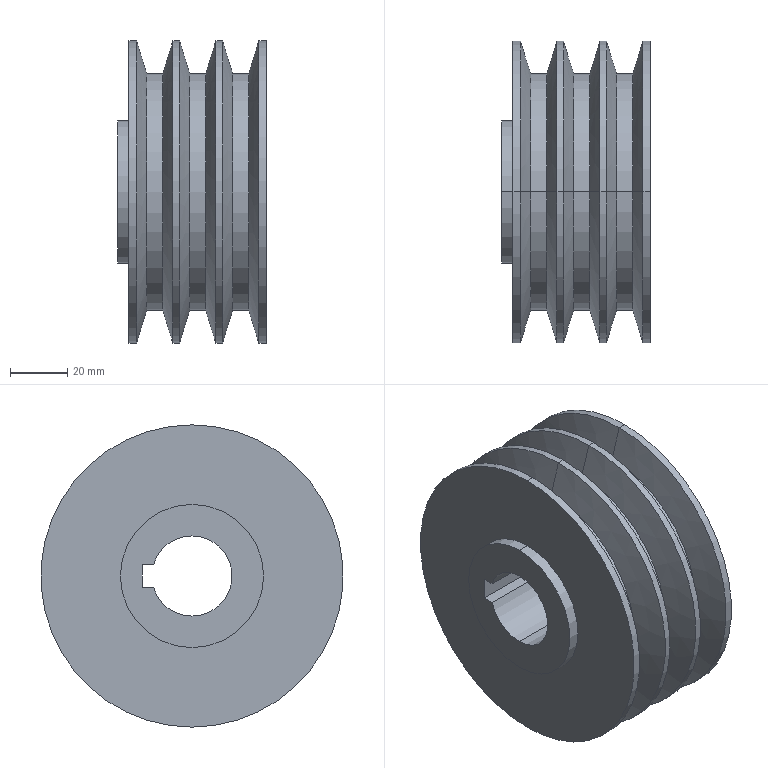Part | SolidWorks | features ICE 2, Revolution 1 | 1 solid | 37 faces | box 52 x 105.5 x 105.5 mm | volume 299364 mm3 | cylinder 19 | cone 12 | plane 6 | commonest cylinder face diameters 105.5 x8 82.6 x6 28 x3 50 x2
STEP:
#1=CARTESIAN_POINT('',(-4.,0.,25.));
#2=VERTEX_POINT('',#1);
#3=CARTESIAN_POINT('',(-4.,0.,-25.));
#4=VERTEX_POINT('',#3);
#5=CARTESIAN_POINT('',(-4.,0.,0.));
#6=DIRECTION('',(-1.,0.,0.));
#7=DIRECTION('',(0.,0.,1.));
#8=AXIS2_PLACEMENT_3D('',#5,#6,#7);
#9=CIRCLE('',#8,25.);
#10=EDGE_CURVE('',#2,#4,#9,.T.);
#11=ORIENTED_EDGE('',*,*,#10,.F.);
#12=CARTESIAN_POINT('',(0.,0.,25.));
#13=VERTEX_POINT('',#12);
#14=CARTESIAN_POINT('',(-4.,0.,25.));
#15=DIRECTION('',(1.,0.,0.));
#16=VECTOR('',#15,1000.);
#17=LINE('',#14,#16);
#18=EDGE_CURVE('',#2,#13,#17,.T.);
#19=ORIENTED_EDGE('',*,*,#18,.T.);
#20=CARTESIAN_POINT('',(0.,0.,-25.));
#21=VERTEX_POINT('',#20);
#22=CARTESIAN_POINT('',(0.,0.,0.));
#23=DIRECTION('',(-1.,0.,0.));
#24=DIRECTION('',(0.,0.,1.));
#25=AXIS2_PLACEMENT_3D('',#22,#23,#24);
#26=CIRCLE('',#25,25.);
#27=EDGE_CURVE('',#13,#21,#26,.T.);
#28=ORIENTED_EDGE('',*,*,#27,.T.);
#29=CARTESIAN_POINT('',(-4.,0.,-25.));
#30=DIRECTION('',(1.,0.,0.));
#31=VECTOR('',#30,1000.);
#32=LINE('',#29,#31);
#33=EDGE_CURVE('',#4,#21,#32,.T.);
#34=ORIENTED_EDGE('',*,*,#33,.F.);
#35=EDGE_LOOP('',(#11,#19,#28,#34));
#36=FACE_OUTER_BOUND('',#35,.T.);
#37=CARTESIAN_POINT('',(-4.,0.,0.));
#38=DIRECTION('',(1.,0.,0.));
#39=DIRECTION('',(0.,0.,-1.));
#40=AXIS2_PLACEMENT_3D('',#37,#38,#39);
#41=CYLINDRICAL_SURFACE('',#40,25.);
#42=ADVANCED_FACE('',(#36),#41,.T.);
#43=CARTESIAN_POINT('',(11.839,0.,-41.3));
#44=VERTEX_POINT('',#43);
#45=CARTESIAN_POINT('',(11.839,0.,41.3));
#46=VERTEX_POINT('',#45);
#47=CARTESIAN_POINT('',(11.839,0.,0.));
#48=DIRECTION('',(1.,0.,0.));
#49=DIRECTION('',(0.,0.,-1.));
#50=AXIS2_PLACEMENT_3D('',#47,#48,#49);
#51=CIRCLE('',#50,41.3);
#52=EDGE_CURVE('',#44,#46,#51,.T.);
#53=ORIENTED_EDGE('',*,*,#52,.T.);
#54=CARTESIAN_POINT('',(15.339,0.,52.75));
#55=VERTEX_POINT('',#54);
#56=CARTESIAN_POINT('',(15.339,0.,52.75));
#57=DIRECTION('',(0.2924,0.,0.9563));
#58=VECTOR('',#57,1000.);
#59=LINE('',#56,#58);
#60=EDGE_CURVE('',#46,#55,#59,.T.);
#61=ORIENTED_EDGE('',*,*,#60,.T.);
#62=CARTESIAN_POINT('',(15.339,0.,-52.75));
#63=VERTEX_POINT('',#62);
#64=CARTESIAN_POINT('',(15.339,0.,0.));
#65=DIRECTION('',(1.,0.,0.));
#66=DIRECTION('',(0.,0.,-1.));
#67=AXIS2_PLACEMENT_3D('',#64,#65,#66);
#68=CIRCLE('',#67,52.75);
#69=EDGE_CURVE('',#63,#55,#68,.T.);
#70=ORIENTED_EDGE('',*,*,#69,.F.);
#71=CARTESIAN_POINT('',(15.339,0.,-52.75));
#72=DIRECTION('',(0.2924,0.,-0.9563));
#73=VECTOR('',#72,1000.);
#74=LINE('',#71,#73);
#75=EDGE_CURVE('',#44,#63,#74,.T.);
#76=ORIENTED_EDGE('',*,*,#75,.F.);
#77=EDGE_LOOP('',(#53,#61,#70,#76));
#78=FACE_OUTER_BOUND('',#77,.T.);
#79=CARTESIAN_POINT('',(15.339,0.,0.));
#80=DIRECTION('',(1.,0.,0.));
#81=DIRECTION('',(0.,0.,-1.));
#82=AXIS2_PLACEMENT_3D('',#79,#80,#81);
#83=CONICAL_SURFACE('',#82,52.75,1.274);
#84=ADVANCED_FACE('',(#78),#83,.T.);
#85=ORIENTED_EDGE('',*,*,#69,.T.);
#86=CARTESIAN_POINT('',(17.659,0.,52.75));
#87=VERTEX_POINT('',#86);
#88=CARTESIAN_POINT('',(0.,0.,52.75));
#89=DIRECTION('',(1.,0.,0.));
#90=VECTOR('',#89,1000.);
#91=LINE('',#88,#90);
#92=EDGE_CURVE('',#55,#87,#91,.T.);
#93=ORIENTED_EDGE('',*,*,#92,.T.);
#94=CARTESIAN_POINT('',(17.659,0.,-52.75));
#95=VERTEX_POINT('',#94);
#96=CARTESIAN_POINT('',(17.659,0.,0.));
#97=DIRECTION('',(1.,0.,0.));
#98=DIRECTION('',(0.,0.,-1.));
#99=AXIS2_PLACEMENT_3D('',#96,#97,#98);
#100=CIRCLE('',#99,52.75);
#101=EDGE_CURVE('',#95,#87,#100,.T.);
#102=ORIENTED_EDGE('',*,*,#101,.F.);
#103=CARTESIAN_POINT('',(0.,0.,-52.75));
#104=DIRECTION('',(1.,0.,0.));
#105=VECTOR('',#104,1000.);
#106=LINE('',#103,#105);
#107=EDGE_CURVE('',#63,#95,#106,.T.);
#108=ORIENTED_EDGE('',*,*,#107,.F.);
#109=EDGE_LOOP('',(#85,#93,#102,#108));
#110=FACE_OUTER_BOUND('',#109,.T.);
#111=CARTESIAN_POINT('',(0.,0.,0.));
#112=DIRECTION('',(1.,0.,0.));
#113=DIRECTION('',(0.,0.,-1.));
#114=AXIS2_PLACEMENT_3D('',#111,#112,#113);
#115=CYLINDRICAL_SURFACE('',#114,52.75);
#116=ADVANCED_FACE('',(#110),#115,.T.);
#117=CARTESIAN_POINT('',(21.16,0.,-41.3));
#118=VERTEX_POINT('',#117);
#119=CARTESIAN_POINT('',(21.16,0.,41.3));
#120=VERTEX_POINT('',#119);
#121=CARTESIAN_POINT('',(21.16,0.,0.));
#122=DIRECTION('',(1.,0.,0.));
#123=DIRECTION('',(0.,0.,-1.));
#124=AXIS2_PLACEMENT_3D('',#121,#122,#123);
#125=CIRCLE('',#124,41.3);
#126=EDGE_CURVE('',#118,#120,#125,.T.);
#127=ORIENTED_EDGE('',*,*,#126,.F.);
#128=CARTESIAN_POINT('',(21.16,0.,-41.3));
#129=DIRECTION('',(-0.2924,0.,-0.9563));
#130=VECTOR('',#129,1000.);
#131=LINE('',#128,#130);
#132=EDGE_CURVE('',#118,#95,#131,.T.);
#133=ORIENTED_EDGE('',*,*,#132,.T.);
#134=ORIENTED_EDGE('',*,*,#101,.T.);
#135=CARTESIAN_POINT('',(21.16,0.,41.3));
#136=DIRECTION('',(-0.2924,0.,0.9563));
#137=VECTOR('',#136,1000.);
#138=LINE('',#135,#137);
#139=EDGE_CURVE('',#120,#87,#138,.T.);
#140=ORIENTED_EDGE('',*,*,#139,.F.);
#141=EDGE_LOOP('',(#127,#133,#134,#140));
#142=FACE_OUTER_BOUND('',#141,.T.);
#143=CARTESIAN_POINT('',(21.16,0.,0.));
#144=DIRECTION('',(-1.,0.,0.));
#145=DIRECTION('',(0.,0.,1.));
#146=AXIS2_PLACEMENT_3D('',#143,#144,#145);
#147=CONICAL_SURFACE('',#146,41.3,1.274);
#148=ADVANCED_FACE('',(#142),#147,.T.);
#149=ORIENTED_EDGE('',*,*,#126,.T.);
#150=CARTESIAN_POINT('',(26.84,0.,41.3));
#151=VERTEX_POINT('',#150);
#152=CARTESIAN_POINT('',(0.,0.,41.3));
#153=DIRECTION('',(1.,0.,0.));
#154=VECTOR('',#153,1000.);
#155=LINE('',#152,#154);
#156=EDGE_CURVE('',#120,#151,#155,.T.);
#157=ORIENTED_EDGE('',*,*,#156,.T.);
#158=CARTESIAN_POINT('',(26.84,0.,-41.3));
#159=VERTEX_POINT('',#158);
#160=CARTESIAN_POINT('',(26.84,0.,0.));
#161=DIRECTION('',(1.,0.,0.));
#162=DIRECTION('',(0.,0.,-1.));
#163=AXIS2_PLACEMENT_3D('',#160,#161,#162);
#164=CIRCLE('',#163,41.3);
#165=EDGE_CURVE('',#159,#151,#164,.T.);
#166=ORIENTED_EDGE('',*,*,#165,.F.);
#167=CARTESIAN_POINT('',(0.,0.,-41.3));
#168=DIRECTION('',(1.,0.,0.));
#169=VECTOR('',#168,1000.);
#170=LINE('',#167,#169);
#171=EDGE_CURVE('',#118,#159,#170,.T.);
#172=ORIENTED_EDGE('',*,*,#171,.F.);
#173=EDGE_LOOP('',(#149,#157,#166,#172));
#174=FACE_OUTER_BOUND('',#173,.T.);
#175=CARTESIAN_POINT('',(0.,0.,0.));
#176=DIRECTION('',(1.,0.,0.));
#177=DIRECTION('',(0.,0.,-1.));
#178=AXIS2_PLACEMENT_3D('',#175,#176,#177);
#179=CYLINDRICAL_SURFACE('',#178,41.3);
#180=ADVANCED_FACE('',(#174),#179,.T.);
#181=ORIENTED_EDGE('',*,*,#165,.T.);
#182=CARTESIAN_POINT('',(30.341,0.,52.75));
#183=VERTEX_POINT('',#182);
#184=CARTESIAN_POINT('',(30.341,0.,52.75));
#185=DIRECTION('',(0.2924,0.,0.9563));
#186=VECTOR('',#185,1000.);
#187=LINE('',#184,#186);
#188=EDGE_CURVE('',#151,#183,#187,.T.);
#189=ORIENTED_EDGE('',*,*,#188,.T.);
#190=CARTESIAN_POINT('',(30.341,0.,-52.75));
#191=VERTEX_POINT('',#190);
#192=CARTESIAN_POINT('',(30.341,0.,0.));
#193=DIRECTION('',(1.,0.,0.));
#194=DIRECTION('',(0.,0.,-1.));
#195=AXIS2_PLACEMENT_3D('',#192,#193,#194);
#196=CIRCLE('',#195,52.75);
#197=EDGE_CURVE('',#191,#183,#196,.T.);
#198=ORIENTED_EDGE('',*,*,#197,.F.);
#199=CARTESIAN_POINT('',(30.341,0.,-52.75));
#200=DIRECTION('',(0.2924,0.,-0.9563));
#201=VECTOR('',#200,1000.);
#202=LINE('',#199,#201);
#203=EDGE_CURVE('',#159,#191,#202,.T.);
#204=ORIENTED_EDGE('',*,*,#203,.F.);
#205=EDGE_LOOP('',(#181,#189,#198,#204));
#206=FACE_OUTER_BOUND('',#205,.T.);
#207=CARTESIAN_POINT('',(30.341,0.,0.));
#208=DIRECTION('',(1.,0.,0.));
#209=DIRECTION('',(0.,0.,-1.));
#210=AXIS2_PLACEMENT_3D('',#207,#208,#209);
#211=CONICAL_SURFACE('',#210,52.75,1.274);
#212=ADVANCED_FACE('',(#206),#211,.T.);
#213=ORIENTED_EDGE('',*,*,#197,.T.);
#214=CARTESIAN_POINT('',(32.661,0.,52.75));
#215=VERTEX_POINT('',#214);
#216=CARTESIAN_POINT('',(0.,0.,52.75));
#217=DIRECTION('',(1.,0.,0.));
#218=VECTOR('',#217,1000.);
#219=LINE('',#216,#218);
#220=EDGE_CURVE('',#183,#215,#219,.T.);
#221=ORIENTED_EDGE('',*,*,#220,.T.);
#222=CARTESIAN_POINT('',(32.661,0.,-52.75));
#223=VERTEX_POINT('',#222);
#224=CARTESIAN_POINT('',(32.661,0.,0.));
#225=DIRECTION('',(1.,0.,0.));
#226=DIRECTION('',(0.,0.,-1.));
#227=AXIS2_PLACEMENT_3D('',#224,#225,#226);
#228=CIRCLE('',#227,52.75);
#229=EDGE_CURVE('',#223,#215,#228,.T.);
#230=ORIENTED_EDGE('',*,*,#229,.F.);
#231=CARTESIAN_POINT('',(0.,0.,-52.75));
#232=DIRECTION('',(1.,0.,0.));
#233=VECTOR('',#232,1000.);
#234=LINE('',#231,#233);
#235=EDGE_CURVE('',#191,#223,#234,.T.);
#236=ORIENTED_EDGE('',*,*,#235,.F.);
#237=EDGE_LOOP('',(#213,#221,#230,#236));
#238=FACE_OUTER_BOUND('',#237,.T.);
#239=CARTESIAN_POINT('',(0.,0.,0.));
#240=DIRECTION('',(1.,0.,0.));
#241=DIRECTION('',(0.,0.,-1.));
#242=AXIS2_PLACEMENT_3D('',#239,#240,#241);
#243=CYLINDRICAL_SURFACE('',#242,52.75);
#244=ADVANCED_FACE('',(#238),#243,.T.);
#245=CARTESIAN_POINT('',(36.161,0.,-41.3));
#246=VERTEX_POINT('',#245);
#247=CARTESIAN_POINT('',(36.161,0.,41.3));
#248=VERTEX_POINT('',#247);
#249=CARTESIAN_POINT('',(36.161,0.,0.));
#250=DIRECTION('',(1.,0.,0.));
#251=DIRECTION('',(0.,0.,-1.));
#252=AXIS2_PLACEMENT_3D('',#249,#250,#251);
#253=CIRCLE('',#252,41.3);
#254=EDGE_CURVE('',#246,#248,#253,.T.);
#255=ORIENTED_EDGE('',*,*,#254,.F.);
#256=CARTESIAN_POINT('',(36.161,0.,-41.3));
#257=DIRECTION('',(-0.2924,0.,-0.9563));
#258=VECTOR('',#257,1000.);
#259=LINE('',#256,#258);
#260=EDGE_CURVE('',#246,#223,#259,.T.);
#261=ORIENTED_EDGE('',*,*,#260,.T.);
#262=ORIENTED_EDGE('',*,*,#229,.T.);
#263=CARTESIAN_POINT('',(36.161,0.,41.3));
#264=DIRECTION('',(-0.2924,0.,0.9563));
#265=VECTOR('',#264,1000.);
#266=LINE('',#263,#265);
#267=EDGE_CURVE('',#248,#215,#266,.T.);
#268=ORIENTED_EDGE('',*,*,#267,.F.);
#269=EDGE_LOOP('',(#255,#261,#262,#268));
#270=FACE_OUTER_BOUND('',#269,.T.);
#271=CARTESIAN_POINT('',(36.161,0.,0.));
#272=DIRECTION('',(-1.,0.,0.));
#273=DIRECTION('',(0.,0.,1.));
#274=AXIS2_PLACEMENT_3D('',#271,#272,#273);
#275=CONICAL_SURFACE('',#274,41.3,1.274);
#276=ADVANCED_FACE('',(#270),#275,.T.);
#277=ORIENTED_EDGE('',*,*,#254,.T.);
#278=CARTESIAN_POINT('',(41.841,0.,41.3));
#279=VERTEX_POINT('',#278);
#280=CARTESIAN_POINT('',(0.,0.,41.3));
#281=DIRECTION('',(1.,0.,0.));
#282=VECTOR('',#281,1000.);
#283=LINE('',#280,#282);
#284=EDGE_CURVE('',#248,#279,#283,.T.);
#285=ORIENTED_EDGE('',*,*,#284,.T.);
#286=CARTESIAN_POINT('',(41.841,0.,-41.3));
#287=VERTEX_POINT('',#286);
#288=CARTESIAN_POINT('',(41.841,0.,0.));
#289=DIRECTION('',(1.,0.,0.));
#290=DIRECTION('',(0.,0.,-1.));
#291=AXIS2_PLACEMENT_3D('',#288,#289,#290);
#292=CIRCLE('',#291,41.3);
#293=EDGE_CURVE('',#287,#279,#292,.T.);
#294=ORIENTED_EDGE('',*,*,#293,.F.);
#295=CARTESIAN_POINT('',(0.,0.,-41.3));
#296=DIRECTION('',(1.,0.,0.));
#297=VECTOR('',#296,1000.);
#298=LINE('',#295,#297);
#299=EDGE_CURVE('',#246,#287,#298,.T.);
#300=ORIENTED_EDGE('',*,*,#299,.F.);
#301=EDGE_LOOP('',(#277,#285,#294,#300));
#302=FACE_OUTER_BOUND('',#301,.T.);
#303=CARTESIAN_POINT('',(0.,0.,0.));
#304=DIRECTION('',(1.,0.,0.));
#305=DIRECTION('',(0.,0.,-1.));
#306=AXIS2_PLACEMENT_3D('',#303,#304,#305);
#307=CYLINDRICAL_SURFACE('',#306,41.3);
#308=ADVANCED_FACE('',(#302),#307,.T.);
#309=ORIENTED_EDGE('',*,*,#293,.T.);
#310=CARTESIAN_POINT('',(45.342,0.,52.75));
#311=VERTEX_POINT('',#310);
#312=CARTESIAN_POINT('',(45.342,0.,52.75));
#313=DIRECTION('',(0.2924,0.,0.9563));
#314=VECTOR('',#313,1000.);
#315=LINE('',#312,#314);
#316=EDGE_CURVE('',#279,#311,#315,.T.);
#317=ORIENTED_EDGE('',*,*,#316,.T.);
#318=CARTESIAN_POINT('',(45.342,0.,-52.75));
#319=VERTEX_POINT('',#318);
#320=CARTESIAN_POINT('',(45.342,0.,0.));
#321=DIRECTION('',(1.,0.,0.));
#322=DIRECTION('',(0.,0.,-1.));
#323=AXIS2_PLACEMENT_3D('',#320,#321,#322);
#324=CIRCLE('',#323,52.75);
#325=EDGE_CURVE('',#319,#311,#324,.T.);
#326=ORIENTED_EDGE('',*,*,#325,.F.);
#327=CARTESIAN_POINT('',(45.342,0.,-52.75));
#328=DIRECTION('',(0.2924,0.,-0.9563));
#329=VECTOR('',#328,1000.);
#330=LINE('',#327,#329);
#331=EDGE_CURVE('',#287,#319,#330,.T.);
#332=ORIENTED_EDGE('',*,*,#331,.F.);
#333=EDGE_LOOP('',(#309,#317,#326,#332));
#334=FACE_OUTER_BOUND('',#333,.T.);
#335=CARTESIAN_POINT('',(45.342,0.,0.));
#336=DIRECTION('',(1.,0.,0.));
#337=DIRECTION('',(0.,0.,-1.));
#338=AXIS2_PLACEMENT_3D('',#335,#336,#337);
#339=CONICAL_SURFACE('',#338,52.75,1.274);
#340=ADVANCED_FACE('',(#334),#339,.T.);
#341=ORIENTED_EDGE('',*,*,#325,.T.);
#342=CARTESIAN_POINT('',(48.,0.,52.75));
#343=VERTEX_POINT('',#342);
#344=CARTESIAN_POINT('',(0.,0.,52.75));
#345=DIRECTION('',(1.,0.,0.));
#346=VECTOR('',#345,1000.);
#347=LINE('',#344,#346);
#348=EDGE_CURVE('',#311,#343,#347,.T.);
#349=ORIENTED_EDGE('',*,*,#348,.T.);
#350=CARTESIAN_POINT('',(48.,0.,-52.75));
#351=VERTEX_POINT('',#350);
#352=CARTESIAN_POINT('',(48.,0.,0.));
#353=DIRECTION('',(1.,0.,0.));
#354=DIRECTION('',(0.,0.,-1.));
#355=AXIS2_PLACEMENT_3D('',#352,#353,#354);
#356=CIRCLE('',#355,52.75);
#357=EDGE_CURVE('',#351,#343,#356,.T.);
#358=ORIENTED_EDGE('',*,*,#357,.F.);
#359=CARTESIAN_POINT('',(0.,0.,-52.75));
#360=DIRECTION('',(1.,0.,0.));
#361=VECTOR('',#360,1000.);
#362=LINE('',#359,#361);
#363=EDGE_CURVE('',#319,#351,#362,.T.);
#364=ORIENTED_EDGE('',*,*,#363,.F.);
#365=EDGE_LOOP('',(#341,#349,#358,#364));
#366=FACE_OUTER_BOUND('',#365,.T.);
#367=CARTESIAN_POINT('',(0.,0.,0.));
#368=DIRECTION('',(1.,0.,0.));
#369=DIRECTION('',(0.,0.,-1.));
#370=AXIS2_PLACEMENT_3D('',#367,#368,#369);
#371=CYLINDRICAL_SURFACE('',#370,52.75);
#372=ADVANCED_FACE('',(#366),#371,.T.);
#373=CARTESIAN_POINT('',(-4.,0.,-14.));
#374=VERTEX_POINT('',#373);
#375=CARTESIAN_POINT('',(-4.,0.,14.));
#376=VERTEX_POINT('',#375);
#377=CARTESIAN_POINT('',(-4.,0.,0.));
#378=DIRECTION('',(-1.,0.,0.));
#379=DIRECTION('',(0.,0.,1.));
#380=AXIS2_PLACEMENT_3D('',#377,#378,#379);
#381=CIRCLE('',#380,14.);
#382=EDGE_CURVE('',#374,#376,#381,.T.);
#383=ORIENTED_EDGE('',*,*,#382,.T.);
#384=CARTESIAN_POINT('',(48.,0.,14.));
#385=VERTEX_POINT('',#384);
#386=CARTESIAN_POINT('',(0.,0.,14.));
#387=DIRECTION('',(1.,0.,0.));
#388=VECTOR('',#387,1000.);
#389=LINE('',#386,#388);
#390=EDGE_CURVE('',#376,#385,#389,.T.);
#391=ORIENTED_EDGE('',*,*,#390,.T.);
#392=CARTESIAN_POINT('',(48.,0.,-14.));
#393=VERTEX_POINT('',#392);
#394=CARTESIAN_POINT('',(48.,0.,0.));
#395=DIRECTION('',(1.,0.,0.));
#396=DIRECTION('',(0.,0.,-1.));
#397=AXIS2_PLACEMENT_3D('',#394,#395,#396);
#398=CIRCLE('',#397,14.);
#399=EDGE_CURVE('',#385,#393,#398,.T.);
#400=ORIENTED_EDGE('',*,*,#399,.T.);
#401=CARTESIAN_POINT('',(0.,0.,-14.));
#402=DIRECTION('',(1.,0.,0.));
#403=VECTOR('',#402,1000.);
#404=LINE('',#401,#403);
#405=EDGE_CURVE('',#374,#393,#404,.T.);
#406=ORIENTED_EDGE('',*,*,#405,.F.);
#407=EDGE_LOOP('',(#383,#391,#400,#406));
#408=FACE_OUTER_BOUND('',#407,.T.);
#409=CARTESIAN_POINT('',(0.,0.,0.));
#410=DIRECTION('',(1.,0.,0.));
#411=DIRECTION('',(0.,0.,-1.));
#412=AXIS2_PLACEMENT_3D('',#409,#410,#411);
#413=CYLINDRICAL_SURFACE('',#412,14.);
#414=ADVANCED_FACE('',(#408),#413,.F.);
#415=CARTESIAN_POINT('',(-4.,13.416,-4.));
#416=VERTEX_POINT('',#415);
#417=CARTESIAN_POINT('',(-4.,0.,0.));
#418=DIRECTION('',(-1.,0.,0.));
#419=DIRECTION('',(0.,0.,1.));
#420=AXIS2_PLACEMENT_3D('',#417,#418,#419);
#421=CIRCLE('',#420,14.);
#422=EDGE_CURVE('',#416,#374,#421,.T.);
#423=ORIENTED_EDGE('',*,*,#422,.T.);
#424=ORIENTED_EDGE('',*,*,#405,.T.);
#425=CARTESIAN_POINT('',(48.,13.416,-4.));
#426=VERTEX_POINT('',#425);
#427=CARTESIAN_POINT('',(48.,0.,0.));
#428=DIRECTION('',(1.,0.,0.));
#429=DIRECTION('',(0.,0.,-1.));
#430=AXIS2_PLACEMENT_3D('',#427,#428,#429);
#431=CIRCLE('',#430,14.);
#432=EDGE_CURVE('',#393,#426,#431,.T.);
#433=ORIENTED_EDGE('',*,*,#432,.T.);
#434=CARTESIAN_POINT('',(0.,13.416,-4.));
#435=DIRECTION('',(-1.,0.,0.));
#436=VECTOR('',#435,1000.);
#437=LINE('',#434,#436);
#438=EDGE_CURVE('',#426,#416,#437,.T.);
#439=ORIENTED_EDGE('',*,*,#438,.T.);
#440=EDGE_LOOP('',(#423,#424,#433,#439));
#441=FACE_OUTER_BOUND('',#440,.T.);
#442=CARTESIAN_POINT('',(0.,0.,0.));
#443=DIRECTION('',(1.,0.,0.));
#444=DIRECTION('',(0.,0.,-1.));
#445=AXIS2_PLACEMENT_3D('',#442,#443,#444);
#446=CYLINDRICAL_SURFACE('',#445,14.);
#447=ADVANCED_FACE('',(#441),#446,.F.);
#448=CARTESIAN_POINT('',(0.,0.,-52.75));
#449=VERTEX_POINT('',#448);
#450=CARTESIAN_POINT('',(0.,0.,52.75));
#451=VERTEX_POINT('',#450);
#452=CARTESIAN_POINT('',(0.,0.,0.));
#453=DIRECTION('',(1.,0.,0.));
#454=DIRECTION('',(0.,0.,-1.));
#455=AXIS2_PLACEMENT_3D('',#452,#453,#454);
#456=CIRCLE('',#455,52.75);
#457=EDGE_CURVE('',#449,#451,#456,.T.);
#458=ORIENTED_EDGE('',*,*,#457,.T.);
#459=CARTESIAN_POINT('',(2.658,0.,52.75));
#460=VERTEX_POINT('',#459);
#461=CARTESIAN_POINT('',(0.,0.,52.75));
#462=DIRECTION('',(1.,0.,0.));
#463=VECTOR('',#462,1000.);
#464=LINE('',#461,#463);
#465=EDGE_CURVE('',#451,#460,#464,.T.);
#466=ORIENTED_EDGE('',*,*,#465,.T.);
#467=CARTESIAN_POINT('',(2.658,0.,-52.75));
#468=VERTEX_POINT('',#467);
#469=CARTESIAN_POINT('',(2.658,0.,0.));
#470=DIRECTION('',(1.,0.,0.));
#471=DIRECTION('',(0.,0.,-1.));
#472=AXIS2_PLACEMENT_3D('',#469,#470,#471);
#473=CIRCLE('',#472,52.75);
#474=EDGE_CURVE('',#468,#460,#473,.T.);
#475=ORIENTED_EDGE('',*,*,#474,.F.);
#476=CARTESIAN_POINT('',(0.,0.,-52.75));
#477=DIRECTION('',(1.,0.,0.));
#478=VECTOR('',#477,1000.);
#479=LINE('',#476,#478);
#480=EDGE_CURVE('',#449,#468,#479,.T.);
#481=ORIENTED_EDGE('',*,*,#480,.F.);
#482=EDGE_LOOP('',(#458,#466,#475,#481));
#483=FACE_OUTER_BOUND('',#482,.T.);
#484=CARTESIAN_POINT('',(0.,0.,0.));
#485=DIRECTION('',(1.,0.,0.));
#486=DIRECTION('',(0.,0.,-1.));
#487=AXIS2_PLACEMENT_3D('',#484,#485,#486);
#488=CYLINDRICAL_SURFACE('',#487,52.75);
#489=ADVANCED_FACE('',(#483),#488,.T.);
#490=CARTESIAN_POINT('',(6.159,0.,-41.3));
#491=VERTEX_POINT('',#490);
#492=CARTESIAN_POINT('',(6.159,0.,41.3));
#493=VERTEX_POINT('',#492);
#494=CARTESIAN_POINT('',(6.159,0.,0.));
#495=DIRECTION('',(1.,0.,0.));
#496=DIRECTION('',(0.,0.,-1.));
#497=AXIS2_PLACEMENT_3D('',#494,#495,#496);
#498=CIRCLE('',#497,41.3);
#499=EDGE_CURVE('',#491,#493,#498,.T.);
#500=ORIENTED_EDGE('',*,*,#499,.F.);
#501=CARTESIAN_POINT('',(6.159,0.,-41.3));
#502=DIRECTION('',(-0.2924,0.,-0.9563));
#503=VECTOR('',#502,1000.);
#504=LINE('',#501,#503);
#505=EDGE_CURVE('',#491,#468,#504,.T.);
#506=ORIENTED_EDGE('',*,*,#505,.T.);
#507=ORIENTED_EDGE('',*,*,#474,.T.);
#508=CARTESIAN_POINT('',(6.159,0.,41.3));
#509=DIRECTION('',(-0.2924,0.,0.9563));
#510=VECTOR('',#509,1000.);
#511=LINE('',#508,#510);
#512=EDGE_CURVE('',#493,#460,#511,.T.);
#513=ORIENTED_EDGE('',*,*,#512,.F.);
#514=EDGE_LOOP('',(#500,#506,#507,#513));
#515=FACE_OUTER_BOUND('',#514,.T.);
#516=CARTESIAN_POINT('',(6.159,0.,0.));
#517=DIRECTION('',(-1.,0.,0.));
#518=DIRECTION('',(0.,0.,1.));
#519=AXIS2_PLACEMENT_3D('',#516,#517,#518);
#520=CONICAL_SURFACE('',#519,41.3,1.274);
#521=ADVANCED_FACE('',(#515),#520,.T.);
#522=ORIENTED_EDGE('',*,*,#499,.T.);
#523=CARTESIAN_POINT('',(0.,0.,41.3));
#524=DIRECTION('',(1.,0.,0.));
#525=VECTOR('',#524,1000.);
#526=LINE('',#523,#525);
#527=EDGE_CURVE('',#493,#46,#526,.T.);
#528=ORIENTED_EDGE('',*,*,#527,.T.);
#529=ORIENTED_EDGE('',*,*,#52,.F.);
#530=CARTESIAN_POINT('',(0.,0.,-41.3));
#531=DIRECTION('',(1.,0.,0.));
#532=VECTOR('',#531,1000.);
#533=LINE('',#530,#532);
#534=EDGE_CURVE('',#491,#44,#533,.T.);
#535=ORIENTED_EDGE('',*,*,#534,.F.);
#536=EDGE_LOOP('',(#522,#528,#529,#535));
#537=FACE_OUTER_BOUND('',#536,.T.);
#538=CARTESIAN_POINT('',(0.,0.,0.));
#539=DIRECTION('',(1.,0.,0.));
#540=DIRECTION('',(0.,0.,-1.));
#541=AXIS2_PLACEMENT_3D('',#538,#539,#540);
#542=CYLINDRICAL_SURFACE('',#541,41.3);
#543=ADVANCED_FACE('',(#537),#542,.T.);
#544=ORIENTED_EDGE('',*,*,#457,.F.);
#545=CARTESIAN_POINT('',(0.,0.,0.));
#546=DIRECTION('',(1.,0.,0.));
#547=DIRECTION('',(0.,0.,-1.));
#548=AXIS2_PLACEMENT_3D('',#545,#546,#547);
#549=CIRCLE('',#548,52.75);
#550=EDGE_CURVE('',#451,#449,#549,.T.);
#551=ORIENTED_EDGE('',*,*,#550,.F.);
#552=EDGE_LOOP('',(#544,#551));
#553=FACE_OUTER_BOUND('',#552,.T.);
#554=CARTESIAN_POINT('',(0.,0.,0.));
#555=DIRECTION('',(-1.,0.,0.));
#556=DIRECTION('',(0.,0.,1.));
#557=AXIS2_PLACEMENT_3D('',#554,#555,#556);
#558=CIRCLE('',#557,25.);
#559=EDGE_CURVE('',#21,#13,#558,.T.);
#560=ORIENTED_EDGE('',*,*,#559,.F.);
#561=ORIENTED_EDGE('',*,*,#27,.F.);
#562=EDGE_LOOP('',(#560,#561));
#563=FACE_BOUND('',#562,.T.);
#564=CARTESIAN_POINT('',(0.,52.75,0.));
#565=DIRECTION('',(-1.,0.,0.));
#566=DIRECTION('',(0.,0.,1.));
#567=AXIS2_PLACEMENT_3D('',#564,#565,#566);
#568=PLANE('',#567);
#569=ADVANCED_FACE('',(#553,#563),#568,.T.);
#570=ORIENTED_EDGE('',*,*,#527,.F.);
#571=CARTESIAN_POINT('',(6.159,0.,0.));
#572=DIRECTION('',(1.,0.,0.));
#573=DIRECTION('',(0.,0.,-1.));
#574=AXIS2_PLACEMENT_3D('',#571,#572,#573);
#575=CIRCLE('',#574,41.3);
#576=EDGE_CURVE('',#493,#491,#575,.T.);
#577=ORIENTED_EDGE('',*,*,#576,.T.);
#578=ORIENTED_EDGE('',*,*,#534,.T.);
#579=CARTESIAN_POINT('',(11.839,0.,0.));
#580=DIRECTION('',(1.,0.,0.));
#581=DIRECTION('',(0.,0.,-1.));
#582=AXIS2_PLACEMENT_3D('',#579,#580,#581);
#583=CIRCLE('',#582,41.3);
#584=EDGE_CURVE('',#46,#44,#583,.T.);
#585=ORIENTED_EDGE('',*,*,#584,.F.);
#586=EDGE_LOOP('',(#570,#577,#578,#585));
#587=FACE_OUTER_BOUND('',#586,.T.);
#588=CARTESIAN_POINT('',(0.,0.,0.));
#589=DIRECTION('',(1.,0.,0.));
#590=DIRECTION('',(0.,0.,-1.));
#591=AXIS2_PLACEMENT_3D('',#588,#589,#590);
#592=CYLINDRICAL_SURFACE('',#591,41.3);
#593=ADVANCED_FACE('',(#587),#592,.T.);
#594=ORIENTED_EDGE('',*,*,#505,.F.);
#595=ORIENTED_EDGE('',*,*,#576,.F.);
#596=ORIENTED_EDGE('',*,*,#512,.T.);
#597=CARTESIAN_POINT('',(2.658,0.,0.));
#598=DIRECTION('',(1.,0.,0.));
#599=DIRECTION('',(0.,0.,-1.));
#600=AXIS2_PLACEMENT_3D('',#597,#598,#599);
#601=CIRCLE('',#600,52.75);
#602=EDGE_CURVE('',#460,#468,#601,.T.);
#603=ORIENTED_EDGE('',*,*,#602,.T.);
#604=EDGE_LOOP('',(#594,#595,#596,#603));
#605=FACE_OUTER_BOUND('',#604,.T.);
#606=CARTESIAN_POINT('',(6.159,0.,0.));
#607=DIRECTION('',(-1.,0.,0.));
#608=DIRECTION('',(0.,0.,1.));
#609=AXIS2_PLACEMENT_3D('',#606,#607,#608);
#610=CONICAL_SURFACE('',#609,41.3,1.274);
#611=ADVANCED_FACE('',(#605),#610,.T.);
#612=ORIENTED_EDGE('',*,*,#465,.F.);
#613=ORIENTED_EDGE('',*,*,#550,.T.);
#614=ORIENTED_EDGE('',*,*,#480,.T.);
#615=ORIENTED_EDGE('',*,*,#602,.F.);
#616=EDGE_LOOP('',(#612,#613,#614,#615));
#617=FACE_OUTER_BOUND('',#616,.T.);
#618=CARTESIAN_POINT('',(0.,0.,0.));
#619=DIRECTION('',(1.,0.,0.));
#620=DIRECTION('',(0.,0.,-1.));
#621=AXIS2_PLACEMENT_3D('',#618,#619,#620);
#622=CYLINDRICAL_SURFACE('',#621,52.75);
#623=ADVANCED_FACE('',(#617),#622,.T.);
#624=ORIENTED_EDGE('',*,*,#390,.F.);
#625=CARTESIAN_POINT('',(-4.,13.416,4.));
#626=VERTEX_POINT('',#625);
#627=CARTESIAN_POINT('',(-4.,0.,0.));
#628=DIRECTION('',(-1.,0.,0.));
#629=DIRECTION('',(0.,0.,1.));
#630=AXIS2_PLACEMENT_3D('',#627,#628,#629);
#631=CIRCLE('',#630,14.);
#632=EDGE_CURVE('',#376,#626,#631,.T.);
#633=ORIENTED_EDGE('',*,*,#632,.T.);
#634=CARTESIAN_POINT('',(48.,13.416,4.));
#635=VERTEX_POINT('',#634);
#636=CARTESIAN_POINT('',(0.,13.416,4.));
#637=DIRECTION('',(1.,0.,0.));
#638=VECTOR('',#637,1000.);
#639=LINE('',#636,#638);
#640=EDGE_CURVE('',#626,#635,#639,.T.);
#641=ORIENTED_EDGE('',*,*,#640,.T.);
#642=CARTESIAN_POINT('',(48.,0.,0.));
#643=DIRECTION('',(1.,0.,0.));
#644=DIRECTION('',(0.,0.,-1.));
#645=AXIS2_PLACEMENT_3D('',#642,#643,#644);
#646=CIRCLE('',#645,14.);
#647=EDGE_CURVE('',#635,#385,#646,.T.);
#648=ORIENTED_EDGE('',*,*,#647,.T.);
#649=EDGE_LOOP('',(#624,#633,#641,#648));
#650=FACE_OUTER_BOUND('',#649,.T.);
#651=CARTESIAN_POINT('',(0.,0.,0.));
#652=DIRECTION('',(1.,0.,0.));
#653=DIRECTION('',(0.,0.,-1.));
#654=AXIS2_PLACEMENT_3D('',#651,#652,#653);
#655=CYLINDRICAL_SURFACE('',#654,14.);
#656=ADVANCED_FACE('',(#650),#655,.F.);
#657=CARTESIAN_POINT('',(48.,17.3,-4.));
#658=VERTEX_POINT('',#657);
#659=CARTESIAN_POINT('',(48.,17.3,-4.));
#660=DIRECTION('',(0.,-1.,0.));
#661=VECTOR('',#660,1000.);
#662=LINE('',#659,#661);
#663=EDGE_CURVE('',#658,#426,#662,.T.);
#664=ORIENTED_EDGE('',*,*,#663,.T.);
#665=ORIENTED_EDGE('',*,*,#432,.F.);
#666=ORIENTED_EDGE('',*,*,#399,.F.);
#667=ORIENTED_EDGE('',*,*,#647,.F.);
#668=CARTESIAN_POINT('',(48.,17.3,4.));
#669=VERTEX_POINT('',#668);
#670=CARTESIAN_POINT('',(48.,17.3,4.));
#671=DIRECTION('',(0.,1.,0.));
#672=VECTOR('',#671,1000.);
#673=LINE('',#670,#672);
#674=EDGE_CURVE('',#635,#669,#673,.T.);
#675=ORIENTED_EDGE('',*,*,#674,.T.);
#676=CARTESIAN_POINT('',(48.,17.3,4.));
#677=DIRECTION('',(0.,0.,-1.));
#678=VECTOR('',#677,1000.);
#679=LINE('',#676,#678);
#680=EDGE_CURVE('',#669,#658,#679,.T.);
#681=ORIENTED_EDGE('',*,*,#680,.T.);
#682=EDGE_LOOP('',(#664,#665,#666,#667,#675,#681));
#683=FACE_BOUND('',#682,.T.);
#684=ORIENTED_EDGE('',*,*,#357,.T.);
#685=CARTESIAN_POINT('',(48.,0.,0.));
#686=DIRECTION('',(1.,0.,0.));
#687=DIRECTION('',(0.,0.,-1.));
#688=AXIS2_PLACEMENT_3D('',#685,#686,#687);
#689=CIRCLE('',#688,52.75);
#690=EDGE_CURVE('',#343,#351,#689,.T.);
#691=ORIENTED_EDGE('',*,*,#690,.T.);
#692=EDGE_LOOP('',(#684,#691));
#693=FACE_OUTER_BOUND('',#692,.T.);
#694=CARTESIAN_POINT('',(48.,14.,0.));
#695=DIRECTION('',(1.,0.,0.));
#696=DIRECTION('',(0.,0.,-1.));
#697=AXIS2_PLACEMENT_3D('',#694,#695,#696);
#698=PLANE('',#697);
#699=ADVANCED_FACE('',(#683,#693),#698,.T.);
#700=ORIENTED_EDGE('',*,*,#348,.F.);
#701=CARTESIAN_POINT('',(45.342,0.,0.));
#702=DIRECTION('',(1.,0.,0.));
#703=DIRECTION('',(0.,0.,-1.));
#704=AXIS2_PLACEMENT_3D('',#701,#702,#703);
#705=CIRCLE('',#704,52.75);
#706=EDGE_CURVE('',#311,#319,#705,.T.);
#707=ORIENTED_EDGE('',*,*,#706,.T.);
#708=ORIENTED_EDGE('',*,*,#363,.T.);
#709=ORIENTED_EDGE('',*,*,#690,.F.);
#710=EDGE_LOOP('',(#700,#707,#708,#709));
#711=FACE_OUTER_BOUND('',#710,.T.);
#712=CARTESIAN_POINT('',(0.,0.,0.));
#713=DIRECTION('',(1.,0.,0.));
#714=DIRECTION('',(0.,0.,-1.));
#715=AXIS2_PLACEMENT_3D('',#712,#713,#714);
#716=CYLINDRICAL_SURFACE('',#715,52.75);
#717=ADVANCED_FACE('',(#711),#716,.T.);
#718=ORIENTED_EDGE('',*,*,#316,.F.);
#719=CARTESIAN_POINT('',(41.841,0.,0.));
#720=DIRECTION('',(1.,0.,0.));
#721=DIRECTION('',(0.,0.,-1.));
#722=AXIS2_PLACEMENT_3D('',#719,#720,#721);
#723=CIRCLE('',#722,41.3);
#724=EDGE_CURVE('',#279,#287,#723,.T.);
#725=ORIENTED_EDGE('',*,*,#724,.T.);
#726=ORIENTED_EDGE('',*,*,#331,.T.);
#727=ORIENTED_EDGE('',*,*,#706,.F.);
#728=EDGE_LOOP('',(#718,#725,#726,#727));
#729=FACE_OUTER_BOUND('',#728,.T.);
#730=CARTESIAN_POINT('',(45.342,0.,0.));
#731=DIRECTION('',(1.,0.,0.));
#732=DIRECTION('',(0.,0.,-1.));
#733=AXIS2_PLACEMENT_3D('',#730,#731,#732);
#734=CONICAL_SURFACE('',#733,52.75,1.274);
#735=ADVANCED_FACE('',(#729),#734,.T.);
#736=ORIENTED_EDGE('',*,*,#284,.F.);
#737=CARTESIAN_POINT('',(36.161,0.,0.));
#738=DIRECTION('',(1.,0.,0.));
#739=DIRECTION('',(0.,0.,-1.));
#740=AXIS2_PLACEMENT_3D('',#737,#738,#739);
#741=CIRCLE('',#740,41.3);
#742=EDGE_CURVE('',#248,#246,#741,.T.);
#743=ORIENTED_EDGE('',*,*,#742,.T.);
#744=ORIENTED_EDGE('',*,*,#299,.T.);
#745=ORIENTED_EDGE('',*,*,#724,.F.);
#746=EDGE_LOOP('',(#736,#743,#744,#745));
#747=FACE_OUTER_BOUND('',#746,.T.);
#748=CARTESIAN_POINT('',(0.,0.,0.));
#749=DIRECTION('',(1.,0.,0.));
#750=DIRECTION('',(0.,0.,-1.));
#751=AXIS2_PLACEMENT_3D('',#748,#749,#750);
#752=CYLINDRICAL_SURFACE('',#751,41.3);
#753=ADVANCED_FACE('',(#747),#752,.T.);
#754=ORIENTED_EDGE('',*,*,#260,.F.);
#755=ORIENTED_EDGE('',*,*,#742,.F.);
#756=ORIENTED_EDGE('',*,*,#267,.T.);
#757=CARTESIAN_POINT('',(32.661,0.,0.));
#758=DIRECTION('',(1.,0.,0.));
#759=DIRECTION('',(0.,0.,-1.));
#760=AXIS2_PLACEMENT_3D('',#757,#758,#759);
#761=CIRCLE('',#760,52.75);
#762=EDGE_CURVE('',#215,#223,#761,.T.);
#763=ORIENTED_EDGE('',*,*,#762,.T.);
#764=EDGE_LOOP('',(#754,#755,#756,#763));
#765=FACE_OUTER_BOUND('',#764,.T.);
#766=CARTESIAN_POINT('',(36.161,0.,0.));
#767=DIRECTION('',(-1.,0.,0.));
#768=DIRECTION('',(0.,0.,1.));
#769=AXIS2_PLACEMENT_3D('',#766,#767,#768);
#770=CONICAL_SURFACE('',#769,41.3,1.274);
#771=ADVANCED_FACE('',(#765),#770,.T.);
#772=ORIENTED_EDGE('',*,*,#220,.F.);
#773=CARTESIAN_POINT('',(30.341,0.,0.));
#774=DIRECTION('',(1.,0.,0.));
#775=DIRECTION('',(0.,0.,-1.));
#776=AXIS2_PLACEMENT_3D('',#773,#774,#775);
#777=CIRCLE('',#776,52.75);
#778=EDGE_CURVE('',#183,#191,#777,.T.);
#779=ORIENTED_EDGE('',*,*,#778,.T.);
#780=ORIENTED_EDGE('',*,*,#235,.T.);
#781=ORIENTED_EDGE('',*,*,#762,.F.);
#782=EDGE_LOOP('',(#772,#779,#780,#781));
#783=FACE_OUTER_BOUND('',#782,.T.);
#784=CARTESIAN_POINT('',(0.,0.,0.));
#785=DIRECTION('',(1.,0.,0.));
#786=DIRECTION('',(0.,0.,-1.));
#787=AXIS2_PLACEMENT_3D('',#784,#785,#786);
#788=CYLINDRICAL_SURFACE('',#787,52.75);
#789=ADVANCED_FACE('',(#783),#788,.T.);
#790=ORIENTED_EDGE('',*,*,#188,.F.);
#791=CARTESIAN_POINT('',(26.84,0.,0.));
#792=DIRECTION('',(1.,0.,0.));
#793=DIRECTION('',(0.,0.,-1.));
#794=AXIS2_PLACEMENT_3D('',#791,#792,#793);
#795=CIRCLE('',#794,41.3);
#796=EDGE_CURVE('',#151,#159,#795,.T.);
#797=ORIENTED_EDGE('',*,*,#796,.T.);
#798=ORIENTED_EDGE('',*,*,#203,.T.);
#799=ORIENTED_EDGE('',*,*,#778,.F.);
#800=EDGE_LOOP('',(#790,#797,#798,#799));
#801=FACE_OUTER_BOUND('',#800,.T.);
#802=CARTESIAN_POINT('',(30.341,0.,0.));
#803=DIRECTION('',(1.,0.,0.));
#804=DIRECTION('',(0.,0.,-1.));
#805=AXIS2_PLACEMENT_3D('',#802,#803,#804);
#806=CONICAL_SURFACE('',#805,52.75,1.274);
#807=ADVANCED_FACE('',(#801),#806,.T.);
#808=ORIENTED_EDGE('',*,*,#156,.F.);
#809=CARTESIAN_POINT('',(21.16,0.,0.));
#810=DIRECTION('',(1.,0.,0.));
#811=DIRECTION('',(0.,0.,-1.));
#812=AXIS2_PLACEMENT_3D('',#809,#810,#811);
#813=CIRCLE('',#812,41.3);
#814=EDGE_CURVE('',#120,#118,#813,.T.);
#815=ORIENTED_EDGE('',*,*,#814,.T.);
#816=ORIENTED_EDGE('',*,*,#171,.T.);
#817=ORIENTED_EDGE('',*,*,#796,.F.);
#818=EDGE_LOOP('',(#808,#815,#816,#817));
#819=FACE_OUTER_BOUND('',#818,.T.);
#820=CARTESIAN_POINT('',(0.,0.,0.));
#821=DIRECTION('',(1.,0.,0.));
#822=DIRECTION('',(0.,0.,-1.));
#823=AXIS2_PLACEMENT_3D('',#820,#821,#822);
#824=CYLINDRICAL_SURFACE('',#823,41.3);
#825=ADVANCED_FACE('',(#819),#824,.T.);
#826=ORIENTED_EDGE('',*,*,#132,.F.);
#827=ORIENTED_EDGE('',*,*,#814,.F.);
#828=ORIENTED_EDGE('',*,*,#139,.T.);
#829=CARTESIAN_POINT('',(17.659,0.,0.));
#830=DIRECTION('',(1.,0.,0.));
#831=DIRECTION('',(0.,0.,-1.));
#832=AXIS2_PLACEMENT_3D('',#829,#830,#831);
#833=CIRCLE('',#832,52.75);
#834=EDGE_CURVE('',#87,#95,#833,.T.);
#835=ORIENTED_EDGE('',*,*,#834,.T.);
#836=EDGE_LOOP('',(#826,#827,#828,#835));
#837=FACE_OUTER_BOUND('',#836,.T.);
#838=CARTESIAN_POINT('',(21.16,0.,0.));
#839=DIRECTION('',(-1.,0.,0.));
#840=DIRECTION('',(0.,0.,1.));
#841=AXIS2_PLACEMENT_3D('',#838,#839,#840);
#842=CONICAL_SURFACE('',#841,41.3,1.274);
#843=ADVANCED_FACE('',(#837),#842,.T.);
#844=ORIENTED_EDGE('',*,*,#92,.F.);
#845=CARTESIAN_POINT('',(15.339,0.,0.));
#846=DIRECTION('',(1.,0.,0.));
#847=DIRECTION('',(0.,0.,-1.));
#848=AXIS2_PLACEMENT_3D('',#845,#846,#847);
#849=CIRCLE('',#848,52.75);
#850=EDGE_CURVE('',#55,#63,#849,.T.);
#851=ORIENTED_EDGE('',*,*,#850,.T.);
#852=ORIENTED_EDGE('',*,*,#107,.T.);
#853=ORIENTED_EDGE('',*,*,#834,.F.);
#854=EDGE_LOOP('',(#844,#851,#852,#853));
#855=FACE_OUTER_BOUND('',#854,.T.);
#856=CARTESIAN_POINT('',(0.,0.,0.));
#857=DIRECTION('',(1.,0.,0.));
#858=DIRECTION('',(0.,0.,-1.));
#859=AXIS2_PLACEMENT_3D('',#856,#857,#858);
#860=CYLINDRICAL_SURFACE('',#859,52.75);
#861=ADVANCED_FACE('',(#855),#860,.T.);
#862=ORIENTED_EDGE('',*,*,#60,.F.);
#863=ORIENTED_EDGE('',*,*,#584,.T.);
#864=ORIENTED_EDGE('',*,*,#75,.T.);
#865=ORIENTED_EDGE('',*,*,#850,.F.);
#866=EDGE_LOOP('',(#862,#863,#864,#865));
#867=FACE_OUTER_BOUND('',#866,.T.);
#868=CARTESIAN_POINT('',(15.339,0.,0.));
#869=DIRECTION('',(1.,0.,0.));
#870=DIRECTION('',(0.,0.,-1.));
#871=AXIS2_PLACEMENT_3D('',#868,#869,#870);
#872=CONICAL_SURFACE('',#871,52.75,1.274);
#873=ADVANCED_FACE('',(#867),#872,.T.);
#874=CARTESIAN_POINT('',(-4.,17.3,-4.));
#875=VERTEX_POINT('',#874);
#876=CARTESIAN_POINT('',(-4.,17.3,-4.));
#877=DIRECTION('',(0.,-1.,0.));
#878=VECTOR('',#877,1000.);
#879=LINE('',#876,#878);
#880=EDGE_CURVE('',#875,#416,#879,.T.);
#881=ORIENTED_EDGE('',*,*,#880,.F.);
#882=CARTESIAN_POINT('',(-4.,17.3,4.));
#883=VERTEX_POINT('',#882);
#884=CARTESIAN_POINT('',(-4.,17.3,4.));
#885=DIRECTION('',(0.,0.,-1.));
#886=VECTOR('',#885,1000.);
#887=LINE('',#884,#886);
#888=EDGE_CURVE('',#883,#875,#887,.T.);
#889=ORIENTED_EDGE('',*,*,#888,.F.);
#890=CARTESIAN_POINT('',(-4.,17.3,4.));
#891=DIRECTION('',(0.,1.,0.));
#892=VECTOR('',#891,1000.);
#893=LINE('',#890,#892);
#894=EDGE_CURVE('',#626,#883,#893,.T.);
#895=ORIENTED_EDGE('',*,*,#894,.F.);
#896=ORIENTED_EDGE('',*,*,#632,.F.);
#897=ORIENTED_EDGE('',*,*,#382,.F.);
#898=ORIENTED_EDGE('',*,*,#422,.F.);
#899=EDGE_LOOP('',(#881,#889,#895,#896,#897,#898));
#900=FACE_BOUND('',#899,.T.);
#901=CARTESIAN_POINT('',(-4.,0.,0.));
#902=DIRECTION('',(-1.,0.,0.));
#903=DIRECTION('',(0.,0.,1.));
#904=AXIS2_PLACEMENT_3D('',#901,#902,#903);
#905=CIRCLE('',#904,25.);
#906=EDGE_CURVE('',#4,#2,#905,.T.);
#907=ORIENTED_EDGE('',*,*,#906,.T.);
#908=ORIENTED_EDGE('',*,*,#10,.T.);
#909=EDGE_LOOP('',(#907,#908));
#910=FACE_OUTER_BOUND('',#909,.T.);
#911=CARTESIAN_POINT('',(-4.,0.,0.));
#912=DIRECTION('',(-1.,0.,0.));
#913=DIRECTION('',(0.,0.,1.));
#914=AXIS2_PLACEMENT_3D('',#911,#912,#913);
#915=PLANE('',#914);
#916=ADVANCED_FACE('',(#900,#910),#915,.T.);
#917=ORIENTED_EDGE('',*,*,#18,.F.);
#918=ORIENTED_EDGE('',*,*,#906,.F.);
#919=ORIENTED_EDGE('',*,*,#33,.T.);
#920=ORIENTED_EDGE('',*,*,#559,.T.);
#921=EDGE_LOOP('',(#917,#918,#919,#920));
#922=FACE_OUTER_BOUND('',#921,.T.);
#923=CARTESIAN_POINT('',(-4.,0.,0.));
#924=DIRECTION('',(1.,0.,0.));
#925=DIRECTION('',(0.,0.,-1.));
#926=AXIS2_PLACEMENT_3D('',#923,#924,#925);
#927=CYLINDRICAL_SURFACE('',#926,25.);
#928=ADVANCED_FACE('',(#922),#927,.T.);
#929=ORIENTED_EDGE('',*,*,#663,.F.);
#930=CARTESIAN_POINT('',(48.001,17.3,-4.));
#931=DIRECTION('',(-1.,0.,0.));
#932=VECTOR('',#931,1000.);
#933=LINE('',#930,#932);
#934=EDGE_CURVE('',#658,#875,#933,.T.);
#935=ORIENTED_EDGE('',*,*,#934,.T.);
#936=ORIENTED_EDGE('',*,*,#880,.T.);
#937=ORIENTED_EDGE('',*,*,#438,.F.);
#938=EDGE_LOOP('',(#929,#935,#936,#937));
#939=FACE_OUTER_BOUND('',#938,.T.);
#940=CARTESIAN_POINT('',(48.001,17.3,-4.));
#941=DIRECTION('',(0.,0.,-1.));
#942=DIRECTION('',(-1.,0.,0.));
#943=AXIS2_PLACEMENT_3D('',#940,#941,#942);
#944=PLANE('',#943);
#945=ADVANCED_FACE('',(#939),#944,.F.);
#946=CARTESIAN_POINT('',(48.001,17.3,4.));
#947=DIRECTION('',(-1.,0.,0.));
#948=VECTOR('',#947,1000.);
#949=LINE('',#946,#948);
#950=EDGE_CURVE('',#669,#883,#949,.T.);
#951=ORIENTED_EDGE('',*,*,#950,.T.);
#952=ORIENTED_EDGE('',*,*,#888,.T.);
#953=ORIENTED_EDGE('',*,*,#934,.F.);
#954=ORIENTED_EDGE('',*,*,#680,.F.);
#955=EDGE_LOOP('',(#951,#952,#953,#954));
#956=FACE_OUTER_BOUND('',#955,.T.);
#957=CARTESIAN_POINT('',(48.001,17.3,4.));
#958=DIRECTION('',(0.,1.,0.));
#959=DIRECTION('',(0.,0.,1.));
#960=AXIS2_PLACEMENT_3D('',#957,#958,#959);
#961=PLANE('',#960);
#962=ADVANCED_FACE('',(#956),#961,.F.);
#963=ORIENTED_EDGE('',*,*,#894,.T.);
#964=ORIENTED_EDGE('',*,*,#950,.F.);
#965=ORIENTED_EDGE('',*,*,#674,.F.);
#966=ORIENTED_EDGE('',*,*,#640,.F.);
#967=EDGE_LOOP('',(#963,#964,#965,#966));
#968=FACE_OUTER_BOUND('',#967,.T.);
#969=CARTESIAN_POINT('',(48.001,17.3,4.));
#970=DIRECTION('',(0.,0.,1.));
#971=DIRECTION('',(1.,0.,0.));
#972=AXIS2_PLACEMENT_3D('',#969,#970,#971);
#973=PLANE('',#972);
#974=ADVANCED_FACE('',(#968),#973,.F.);
#975=CLOSED_SHELL('',(#42,#84,#116,#148,#180,#212,#244,#276,#308,#340,#372,#414,#447,#489,#521,#543,#569,#593,#611,#623,#656,#699,#717,#735,#753,#771,#789,#807,#825,#843,#861,#873,#916,#928,#945,#962,#974));
#976=MANIFOLD_SOLID_BREP('',#975);
#977=CARTESIAN_POINT('',(0.,0.,0.));
#978=DIRECTION('',(0.,0.,1.));
#979=DIRECTION('',(1.,0.,0.));
#980=AXIS2_PLACEMENT_3D('',#977,#978,#979);
#981=(LENGTH_UNIT()NAMED_UNIT(*)SI_UNIT(.MILLI.,.METRE.));
#982=UNCERTAINTY_MEASURE_WITH_UNIT(LENGTH_MEASURE(0.00001),#981,'','');
#983=(NAMED_UNIT(*)PLANE_ANGLE_UNIT()SI_UNIT($,.RADIAN.));
#984=(NAMED_UNIT(*)SI_UNIT($,.STERADIAN.)SOLID_ANGLE_UNIT());
#985=(GEOMETRIC_REPRESENTATION_CONTEXT(3)GLOBAL_UNCERTAINTY_ASSIGNED_CONTEXT((#982))GLOBAL_UNIT_ASSIGNED_CONTEXT((#981,#983,#984))REPRESENTATION_CONTEXT('',''));
#986=ADVANCED_BREP_SHAPE_REPRESENTATION('',(#976,#980),#985);